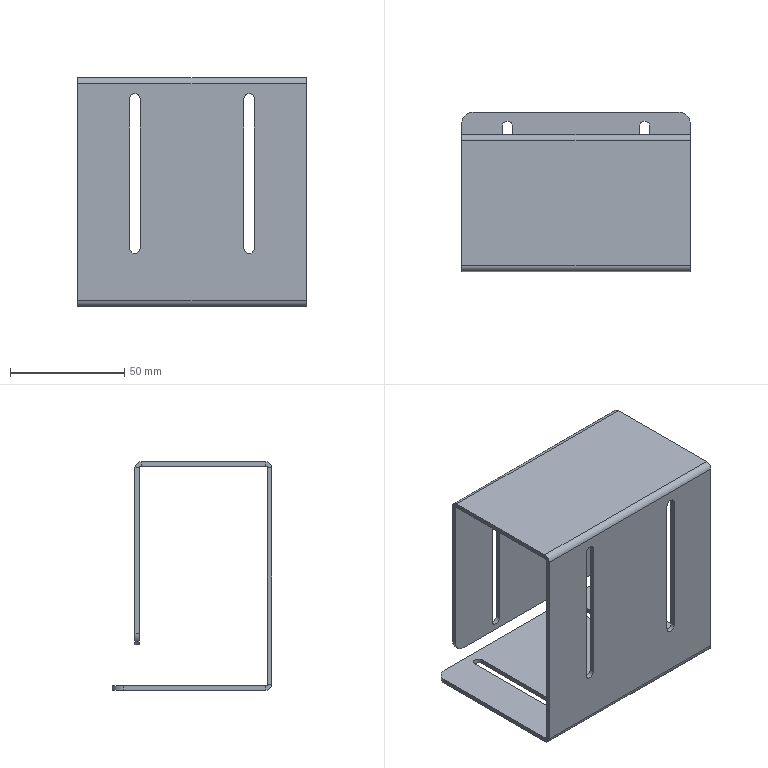Part | SolidWorks | features EdgeFlange 3, HoleWzd 2, Fillet 1, FlatPattern 1, SMBaseFlange 1, SheetMetal 1 | 1 solid | 62 faces | box 100 x 70 x 100 mm | volume 56762 mm3 | plane 36 | cylinder 26 | commonest cylinder face diameters 4.5 x16 10 x4 1.473 x3 5.473 x3